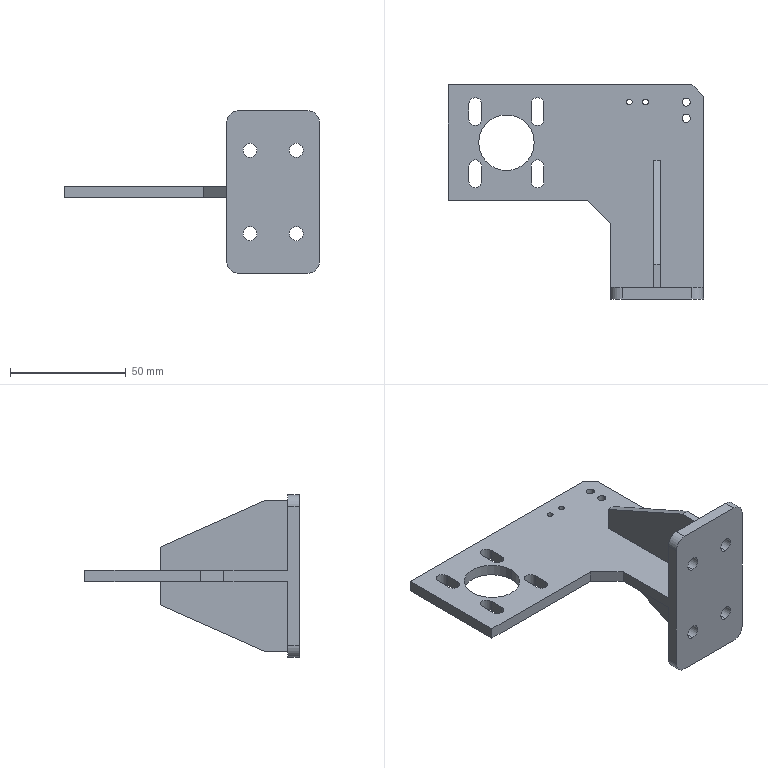Part | STEP file | Lead screw guide rail connecting plate split 1V1.201001 | 1 solid | 62 faces | box 110 x 92.5 x 70 mm | volume 52117 mm3 | plane 32 | cylinder 30 | commonest cylinder face diameters 5.5 x8 6 x8 2.5 x4 3.5 x4 10 x4 24 x2